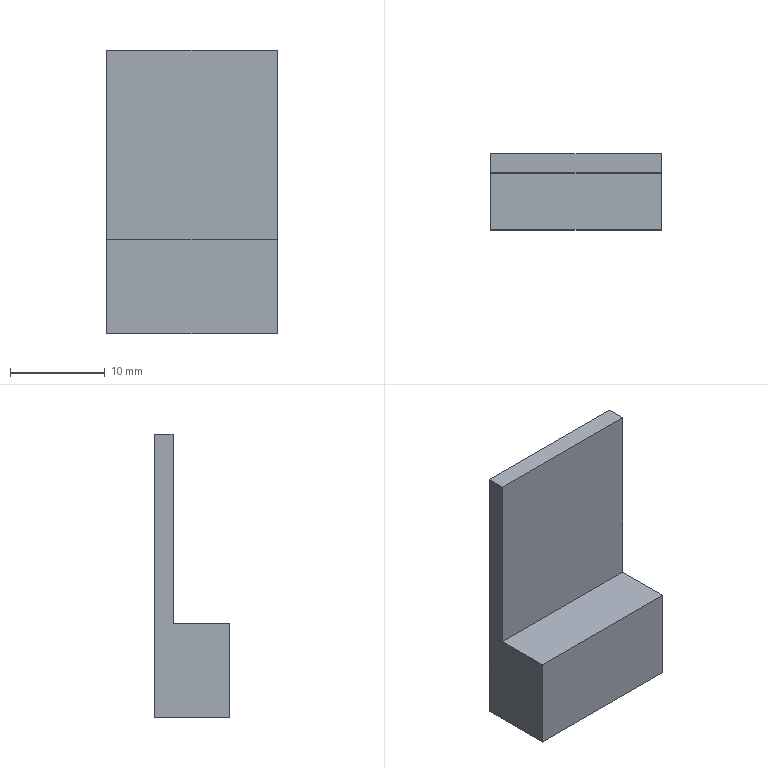Part | SolidWorks | features 3DProfileFeature 1, Extrusion 1, HoleWzd 1, ICE 1, MirrorPattern 1 | 1 solid | 20 faces | box 18 x 8 x 30 mm | volume 2093 mm3 | cone 8 | plane 8 | cylinder 4 | commonest cylinder face diameters 2.5 x4
STEP:
#1=CARTESIAN_POINT('',(-3.75,0.,0.275));
#2=VERTEX_POINT('',#1);
#3=CARTESIAN_POINT('',(-6.25,0.,0.275));
#4=VERTEX_POINT('',#3);
#5=CARTESIAN_POINT('',(-5.,0.,0.275));
#6=DIRECTION('',(0.,0.,-1.));
#7=DIRECTION('',(-1.,0.,0.));
#8=AXIS2_PLACEMENT_3D('',#5,#6,#7);
#9=CIRCLE('',#8,1.25);
#10=EDGE_CURVE('',#2,#4,#9,.T.);
#11=ORIENTED_EDGE('',*,*,#10,.F.);
#12=CARTESIAN_POINT('',(-3.475,0.,0.));
#13=VERTEX_POINT('',#12);
#14=CARTESIAN_POINT('',(-3.475,0.,0.));
#15=DIRECTION('',(0.7071,0.,-0.7071));
#16=VECTOR('',#15,1000.);
#17=LINE('',#14,#16);
#18=EDGE_CURVE('',#2,#13,#17,.T.);
#19=ORIENTED_EDGE('',*,*,#18,.T.);
#20=CARTESIAN_POINT('',(-6.525,0.,0.));
#21=VERTEX_POINT('',#20);
#22=CARTESIAN_POINT('',(-5.,0.,0.));
#23=DIRECTION('',(0.,0.,-1.));
#24=DIRECTION('',(-1.,0.,0.));
#25=AXIS2_PLACEMENT_3D('',#22,#23,#24);
#26=CIRCLE('',#25,1.525);
#27=EDGE_CURVE('',#13,#21,#26,.T.);
#28=ORIENTED_EDGE('',*,*,#27,.T.);
#29=CARTESIAN_POINT('',(-6.525,0.,0.));
#30=DIRECTION('',(-0.7071,0.,-0.7071));
#31=VECTOR('',#30,1000.);
#32=LINE('',#29,#31);
#33=EDGE_CURVE('',#4,#21,#32,.T.);
#34=ORIENTED_EDGE('',*,*,#33,.F.);
#35=EDGE_LOOP('',(#11,#19,#28,#34));
#36=FACE_OUTER_BOUND('',#35,.T.);
#37=CARTESIAN_POINT('',(-5.,0.,0.));
#38=DIRECTION('',(0.,0.,-1.));
#39=DIRECTION('',(-1.,0.,0.));
#40=AXIS2_PLACEMENT_3D('',#37,#38,#39);
#41=CONICAL_SURFACE('',#40,1.525,0.7854);
#42=ADVANCED_FACE('',(#36),#41,.F.);
#43=CARTESIAN_POINT('',(-3.75,0.,6.5));
#44=VERTEX_POINT('',#43);
#45=CARTESIAN_POINT('',(-6.25,0.,6.5));
#46=VERTEX_POINT('',#45);
#47=CARTESIAN_POINT('',(-5.,0.,6.5));
#48=DIRECTION('',(0.,0.,-1.));
#49=DIRECTION('',(-1.,0.,0.));
#50=AXIS2_PLACEMENT_3D('',#47,#48,#49);
#51=CIRCLE('',#50,1.25);
#52=EDGE_CURVE('',#44,#46,#51,.T.);
#53=ORIENTED_EDGE('',*,*,#52,.F.);
#54=CARTESIAN_POINT('',(-3.75,0.,0.));
#55=DIRECTION('',(0.,0.,-1.));
#56=VECTOR('',#55,1000.);
#57=LINE('',#54,#56);
#58=EDGE_CURVE('',#44,#2,#57,.T.);
#59=ORIENTED_EDGE('',*,*,#58,.T.);
#60=ORIENTED_EDGE('',*,*,#10,.T.);
#61=CARTESIAN_POINT('',(-6.25,0.,0.));
#62=DIRECTION('',(0.,0.,-1.));
#63=VECTOR('',#62,1000.);
#64=LINE('',#61,#63);
#65=EDGE_CURVE('',#46,#4,#64,.T.);
#66=ORIENTED_EDGE('',*,*,#65,.F.);
#67=EDGE_LOOP('',(#53,#59,#60,#66));
#68=FACE_OUTER_BOUND('',#67,.T.);
#69=CARTESIAN_POINT('',(-5.,0.,0.));
#70=DIRECTION('',(0.,0.,-1.));
#71=DIRECTION('',(-1.,0.,0.));
#72=AXIS2_PLACEMENT_3D('',#69,#70,#71);
#73=CYLINDRICAL_SURFACE('',#72,1.25);
#74=ADVANCED_FACE('',(#68),#73,.F.);
#75=CARTESIAN_POINT('',(-5.,0.,7.251));
#76=VERTEX_POINT('',#75);
#77=CARTESIAN_POINT('',(-6.25,0.,6.5));
#78=DIRECTION('',(-0.8572,0.,-0.515));
#79=VECTOR('',#78,1000.);
#80=LINE('',#77,#79);
#81=EDGE_CURVE('',#76,#46,#80,.T.);
#82=ORIENTED_EDGE('',*,*,#81,.F.);
#83=CARTESIAN_POINT('',(-3.75,0.,6.5));
#84=DIRECTION('',(0.8572,0.,-0.515));
#85=VECTOR('',#84,1000.);
#86=LINE('',#83,#85);
#87=EDGE_CURVE('',#76,#44,#86,.T.);
#88=ORIENTED_EDGE('',*,*,#87,.T.);
#89=ORIENTED_EDGE('',*,*,#52,.T.);
#90=EDGE_LOOP('',(#82,#88,#89));
#91=FACE_OUTER_BOUND('',#90,.T.);
#92=CARTESIAN_POINT('',(-5.,0.,6.5));
#93=DIRECTION('',(0.,0.,-1.));
#94=DIRECTION('',(-1.,0.,0.));
#95=AXIS2_PLACEMENT_3D('',#92,#93,#94);
#96=CONICAL_SURFACE('',#95,1.25,1.03);
#97=ADVANCED_FACE('',(#91),#96,.F.);
#98=CARTESIAN_POINT('',(6.25,0.,0.275));
#99=VERTEX_POINT('',#98);
#100=CARTESIAN_POINT('',(3.75,0.,0.275));
#101=VERTEX_POINT('',#100);
#102=CARTESIAN_POINT('',(5.,0.,0.275));
#103=DIRECTION('',(0.,0.,-1.));
#104=DIRECTION('',(-1.,0.,0.));
#105=AXIS2_PLACEMENT_3D('',#102,#103,#104);
#106=CIRCLE('',#105,1.25);
#107=EDGE_CURVE('',#99,#101,#106,.T.);
#108=ORIENTED_EDGE('',*,*,#107,.F.);
#109=CARTESIAN_POINT('',(6.525,0.,0.));
#110=VERTEX_POINT('',#109);
#111=CARTESIAN_POINT('',(6.525,0.,0.));
#112=DIRECTION('',(0.7071,0.,-0.7071));
#113=VECTOR('',#112,1000.);
#114=LINE('',#111,#113);
#115=EDGE_CURVE('',#99,#110,#114,.T.);
#116=ORIENTED_EDGE('',*,*,#115,.T.);
#117=CARTESIAN_POINT('',(3.475,0.,0.));
#118=VERTEX_POINT('',#117);
#119=CARTESIAN_POINT('',(5.,0.,0.));
#120=DIRECTION('',(0.,0.,-1.));
#121=DIRECTION('',(-1.,0.,0.));
#122=AXIS2_PLACEMENT_3D('',#119,#120,#121);
#123=CIRCLE('',#122,1.525);
#124=EDGE_CURVE('',#110,#118,#123,.T.);
#125=ORIENTED_EDGE('',*,*,#124,.T.);
#126=CARTESIAN_POINT('',(3.475,0.,0.));
#127=DIRECTION('',(-0.7071,0.,-0.7071));
#128=VECTOR('',#127,1000.);
#129=LINE('',#126,#128);
#130=EDGE_CURVE('',#101,#118,#129,.T.);
#131=ORIENTED_EDGE('',*,*,#130,.F.);
#132=EDGE_LOOP('',(#108,#116,#125,#131));
#133=FACE_OUTER_BOUND('',#132,.T.);
#134=CARTESIAN_POINT('',(5.,0.,0.));
#135=DIRECTION('',(0.,0.,-1.));
#136=DIRECTION('',(-1.,0.,0.));
#137=AXIS2_PLACEMENT_3D('',#134,#135,#136);
#138=CONICAL_SURFACE('',#137,1.525,0.7854);
#139=ADVANCED_FACE('',(#133),#138,.F.);
#140=CARTESIAN_POINT('',(6.25,0.,6.5));
#141=VERTEX_POINT('',#140);
#142=CARTESIAN_POINT('',(3.75,0.,6.5));
#143=VERTEX_POINT('',#142);
#144=CARTESIAN_POINT('',(5.,0.,6.5));
#145=DIRECTION('',(0.,0.,-1.));
#146=DIRECTION('',(-1.,0.,0.));
#147=AXIS2_PLACEMENT_3D('',#144,#145,#146);
#148=CIRCLE('',#147,1.25);
#149=EDGE_CURVE('',#141,#143,#148,.T.);
#150=ORIENTED_EDGE('',*,*,#149,.F.);
#151=CARTESIAN_POINT('',(6.25,0.,0.));
#152=DIRECTION('',(0.,0.,-1.));
#153=VECTOR('',#152,1000.);
#154=LINE('',#151,#153);
#155=EDGE_CURVE('',#141,#99,#154,.T.);
#156=ORIENTED_EDGE('',*,*,#155,.T.);
#157=ORIENTED_EDGE('',*,*,#107,.T.);
#158=CARTESIAN_POINT('',(3.75,0.,0.));
#159=DIRECTION('',(0.,0.,-1.));
#160=VECTOR('',#159,1000.);
#161=LINE('',#158,#160);
#162=EDGE_CURVE('',#143,#101,#161,.T.);
#163=ORIENTED_EDGE('',*,*,#162,.F.);
#164=EDGE_LOOP('',(#150,#156,#157,#163));
#165=FACE_OUTER_BOUND('',#164,.T.);
#166=CARTESIAN_POINT('',(5.,0.,0.));
#167=DIRECTION('',(0.,0.,-1.));
#168=DIRECTION('',(-1.,0.,0.));
#169=AXIS2_PLACEMENT_3D('',#166,#167,#168);
#170=CYLINDRICAL_SURFACE('',#169,1.25);
#171=ADVANCED_FACE('',(#165),#170,.F.);
#172=CARTESIAN_POINT('',(5.,0.,7.251));
#173=VERTEX_POINT('',#172);
#174=CARTESIAN_POINT('',(3.75,0.,6.5));
#175=DIRECTION('',(-0.8572,0.,-0.515));
#176=VECTOR('',#175,1000.);
#177=LINE('',#174,#176);
#178=EDGE_CURVE('',#173,#143,#177,.T.);
#179=ORIENTED_EDGE('',*,*,#178,.F.);
#180=CARTESIAN_POINT('',(6.25,0.,6.5));
#181=DIRECTION('',(0.8572,0.,-0.515));
#182=VECTOR('',#181,1000.);
#183=LINE('',#180,#182);
#184=EDGE_CURVE('',#173,#141,#183,.T.);
#185=ORIENTED_EDGE('',*,*,#184,.T.);
#186=ORIENTED_EDGE('',*,*,#149,.T.);
#187=EDGE_LOOP('',(#179,#185,#186));
#188=FACE_OUTER_BOUND('',#187,.T.);
#189=CARTESIAN_POINT('',(5.,0.,6.5));
#190=DIRECTION('',(0.,0.,-1.));
#191=DIRECTION('',(-1.,0.,0.));
#192=AXIS2_PLACEMENT_3D('',#189,#190,#191);
#193=CONICAL_SURFACE('',#192,1.25,1.03);
#194=ADVANCED_FACE('',(#188),#193,.F.);
#195=CARTESIAN_POINT('',(-9.,2.,10.));
#196=VERTEX_POINT('',#195);
#197=CARTESIAN_POINT('',(9.,2.,10.));
#198=VERTEX_POINT('',#197);
#199=CARTESIAN_POINT('',(-9.,2.,10.));
#200=DIRECTION('',(1.,0.,0.));
#201=VECTOR('',#200,1000.);
#202=LINE('',#199,#201);
#203=EDGE_CURVE('',#196,#198,#202,.T.);
#204=ORIENTED_EDGE('',*,*,#203,.F.);
#205=CARTESIAN_POINT('',(-9.,-4.,10.));
#206=VERTEX_POINT('',#205);
#207=CARTESIAN_POINT('',(-9.,-4.,10.));
#208=DIRECTION('',(0.,-1.,0.));
#209=VECTOR('',#208,1000.);
#210=LINE('',#207,#209);
#211=EDGE_CURVE('',#196,#206,#210,.T.);
#212=ORIENTED_EDGE('',*,*,#211,.T.);
#213=CARTESIAN_POINT('',(9.,-4.,10.));
#214=VERTEX_POINT('',#213);
#215=CARTESIAN_POINT('',(-9.,-4.,10.));
#216=DIRECTION('',(1.,0.,0.));
#217=VECTOR('',#216,1000.);
#218=LINE('',#215,#217);
#219=EDGE_CURVE('',#206,#214,#218,.T.);
#220=ORIENTED_EDGE('',*,*,#219,.T.);
#221=CARTESIAN_POINT('',(9.,-4.,10.));
#222=DIRECTION('',(0.,1.,0.));
#223=VECTOR('',#222,1000.);
#224=LINE('',#221,#223);
#225=EDGE_CURVE('',#214,#198,#224,.T.);
#226=ORIENTED_EDGE('',*,*,#225,.T.);
#227=EDGE_LOOP('',(#204,#212,#220,#226));
#228=FACE_OUTER_BOUND('',#227,.T.);
#229=CARTESIAN_POINT('',(0.,0.,10.));
#230=DIRECTION('',(0.,0.,-1.));
#231=DIRECTION('',(-1.,0.,0.));
#232=AXIS2_PLACEMENT_3D('',#229,#230,#231);
#233=PLANE('',#232);
#234=ADVANCED_FACE('',(#228),#233,.F.);
#235=CARTESIAN_POINT('',(9.,-4.,0.));
#236=VERTEX_POINT('',#235);
#237=CARTESIAN_POINT('',(9.,4.,0.));
#238=VERTEX_POINT('',#237);
#239=CARTESIAN_POINT('',(9.,-4.,0.));
#240=DIRECTION('',(0.,1.,0.));
#241=VECTOR('',#240,1000.);
#242=LINE('',#239,#241);
#243=EDGE_CURVE('',#236,#238,#242,.T.);
#244=ORIENTED_EDGE('',*,*,#243,.T.);
#245=CARTESIAN_POINT('',(9.,4.,30.));
#246=VERTEX_POINT('',#245);
#247=CARTESIAN_POINT('',(9.,4.,10.));
#248=DIRECTION('',(0.,0.,-1.));
#249=VECTOR('',#248,1000.);
#250=LINE('',#247,#249);
#251=EDGE_CURVE('',#246,#238,#250,.T.);
#252=ORIENTED_EDGE('',*,*,#251,.F.);
#253=CARTESIAN_POINT('',(9.,2.,30.));
#254=VERTEX_POINT('',#253);
#255=CARTESIAN_POINT('',(9.,4.,30.));
#256=DIRECTION('',(0.,1.,0.));
#257=VECTOR('',#256,1000.);
#258=LINE('',#255,#257);
#259=EDGE_CURVE('',#254,#246,#258,.T.);
#260=ORIENTED_EDGE('',*,*,#259,.F.);
#261=CARTESIAN_POINT('',(9.,2.,30.));
#262=DIRECTION('',(0.,0.,-1.));
#263=VECTOR('',#262,1000.);
#264=LINE('',#261,#263);
#265=EDGE_CURVE('',#254,#198,#264,.T.);
#266=ORIENTED_EDGE('',*,*,#265,.T.);
#267=ORIENTED_EDGE('',*,*,#225,.F.);
#268=CARTESIAN_POINT('',(9.,-4.,10.));
#269=DIRECTION('',(0.,0.,-1.));
#270=VECTOR('',#269,1000.);
#271=LINE('',#268,#270);
#272=EDGE_CURVE('',#214,#236,#271,.T.);
#273=ORIENTED_EDGE('',*,*,#272,.T.);
#274=EDGE_LOOP('',(#244,#252,#260,#266,#267,#273));
#275=FACE_OUTER_BOUND('',#274,.T.);
#276=CARTESIAN_POINT('',(9.,-4.,10.));
#277=DIRECTION('',(-1.,0.,0.));
#278=DIRECTION('',(0.,0.,1.));
#279=AXIS2_PLACEMENT_3D('',#276,#277,#278);
#280=PLANE('',#279);
#281=ADVANCED_FACE('',(#275),#280,.F.);
#282=CARTESIAN_POINT('',(-9.,4.,0.));
#283=VERTEX_POINT('',#282);
#284=CARTESIAN_POINT('',(-9.,4.,0.));
#285=DIRECTION('',(-1.,0.,0.));
#286=VECTOR('',#285,1000.);
#287=LINE('',#284,#286);
#288=EDGE_CURVE('',#238,#283,#287,.T.);
#289=ORIENTED_EDGE('',*,*,#288,.T.);
#290=CARTESIAN_POINT('',(-9.,4.,30.));
#291=VERTEX_POINT('',#290);
#292=CARTESIAN_POINT('',(-9.,4.,10.));
#293=DIRECTION('',(0.,0.,-1.));
#294=VECTOR('',#293,1000.);
#295=LINE('',#292,#294);
#296=EDGE_CURVE('',#291,#283,#295,.T.);
#297=ORIENTED_EDGE('',*,*,#296,.F.);
#298=CARTESIAN_POINT('',(-9.,4.,30.));
#299=DIRECTION('',(-1.,0.,0.));
#300=VECTOR('',#299,1000.);
#301=LINE('',#298,#300);
#302=EDGE_CURVE('',#246,#291,#301,.T.);
#303=ORIENTED_EDGE('',*,*,#302,.F.);
#304=ORIENTED_EDGE('',*,*,#251,.T.);
#305=EDGE_LOOP('',(#289,#297,#303,#304));
#306=FACE_OUTER_BOUND('',#305,.T.);
#307=CARTESIAN_POINT('',(-9.,4.,10.));
#308=DIRECTION('',(0.,-1.,0.));
#309=DIRECTION('',(0.,0.,-1.));
#310=AXIS2_PLACEMENT_3D('',#307,#308,#309);
#311=PLANE('',#310);
#312=ADVANCED_FACE('',(#306),#311,.F.);
#313=CARTESIAN_POINT('',(-9.,-4.,0.));
#314=VERTEX_POINT('',#313);
#315=CARTESIAN_POINT('',(-9.,-4.,0.));
#316=DIRECTION('',(0.,-1.,0.));
#317=VECTOR('',#316,1000.);
#318=LINE('',#315,#317);
#319=EDGE_CURVE('',#283,#314,#318,.T.);
#320=ORIENTED_EDGE('',*,*,#319,.T.);
#321=CARTESIAN_POINT('',(-9.,-4.,10.));
#322=DIRECTION('',(0.,0.,-1.));
#323=VECTOR('',#322,1000.);
#324=LINE('',#321,#323);
#325=EDGE_CURVE('',#206,#314,#324,.T.);
#326=ORIENTED_EDGE('',*,*,#325,.F.);
#327=ORIENTED_EDGE('',*,*,#211,.F.);
#328=CARTESIAN_POINT('',(-9.,2.,30.));
#329=VERTEX_POINT('',#328);
#330=CARTESIAN_POINT('',(-9.,2.,30.));
#331=DIRECTION('',(0.,0.,-1.));
#332=VECTOR('',#331,1000.);
#333=LINE('',#330,#332);
#334=EDGE_CURVE('',#329,#196,#333,.T.);
#335=ORIENTED_EDGE('',*,*,#334,.F.);
#336=CARTESIAN_POINT('',(-9.,4.,30.));
#337=DIRECTION('',(0.,-1.,0.));
#338=VECTOR('',#337,1000.);
#339=LINE('',#336,#338);
#340=EDGE_CURVE('',#291,#329,#339,.T.);
#341=ORIENTED_EDGE('',*,*,#340,.F.);
#342=ORIENTED_EDGE('',*,*,#296,.T.);
#343=EDGE_LOOP('',(#320,#326,#327,#335,#341,#342));
#344=FACE_OUTER_BOUND('',#343,.T.);
#345=CARTESIAN_POINT('',(-9.,-4.,10.));
#346=DIRECTION('',(1.,0.,0.));
#347=DIRECTION('',(0.,0.,-1.));
#348=AXIS2_PLACEMENT_3D('',#345,#346,#347);
#349=PLANE('',#348);
#350=ADVANCED_FACE('',(#344),#349,.F.);
#351=CARTESIAN_POINT('',(-9.,-4.,0.));
#352=DIRECTION('',(1.,0.,0.));
#353=VECTOR('',#352,1000.);
#354=LINE('',#351,#353);
#355=EDGE_CURVE('',#314,#236,#354,.T.);
#356=ORIENTED_EDGE('',*,*,#355,.T.);
#357=ORIENTED_EDGE('',*,*,#272,.F.);
#358=ORIENTED_EDGE('',*,*,#219,.F.);
#359=ORIENTED_EDGE('',*,*,#325,.T.);
#360=EDGE_LOOP('',(#356,#357,#358,#359));
#361=FACE_OUTER_BOUND('',#360,.T.);
#362=CARTESIAN_POINT('',(-9.,-4.,10.));
#363=DIRECTION('',(0.,1.,0.));
#364=DIRECTION('',(0.,0.,1.));
#365=AXIS2_PLACEMENT_3D('',#362,#363,#364);
#366=PLANE('',#365);
#367=ADVANCED_FACE('',(#361),#366,.F.);
#368=CARTESIAN_POINT('',(-5.,0.,0.));
#369=DIRECTION('',(0.,0.,-1.));
#370=DIRECTION('',(-1.,0.,0.));
#371=AXIS2_PLACEMENT_3D('',#368,#369,#370);
#372=CIRCLE('',#371,1.525);
#373=EDGE_CURVE('',#21,#13,#372,.T.);
#374=ORIENTED_EDGE('',*,*,#373,.F.);
#375=ORIENTED_EDGE('',*,*,#27,.F.);
#376=EDGE_LOOP('',(#374,#375));
#377=FACE_BOUND('',#376,.T.);
#378=CARTESIAN_POINT('',(5.,0.,0.));
#379=DIRECTION('',(0.,0.,-1.));
#380=DIRECTION('',(-1.,0.,0.));
#381=AXIS2_PLACEMENT_3D('',#378,#379,#380);
#382=CIRCLE('',#381,1.525);
#383=EDGE_CURVE('',#118,#110,#382,.T.);
#384=ORIENTED_EDGE('',*,*,#383,.F.);
#385=ORIENTED_EDGE('',*,*,#124,.F.);
#386=EDGE_LOOP('',(#384,#385));
#387=FACE_BOUND('',#386,.T.);
#388=ORIENTED_EDGE('',*,*,#243,.F.);
#389=ORIENTED_EDGE('',*,*,#355,.F.);
#390=ORIENTED_EDGE('',*,*,#319,.F.);
#391=ORIENTED_EDGE('',*,*,#288,.F.);
#392=EDGE_LOOP('',(#388,#389,#390,#391));
#393=FACE_OUTER_BOUND('',#392,.T.);
#394=CARTESIAN_POINT('',(0.,0.,0.));
#395=DIRECTION('',(0.,0.,-1.));
#396=DIRECTION('',(-1.,0.,0.));
#397=AXIS2_PLACEMENT_3D('',#394,#395,#396);
#398=PLANE('',#397);
#399=ADVANCED_FACE('',(#377,#387,#393),#398,.T.);
#400=ORIENTED_EDGE('',*,*,#203,.T.);
#401=ORIENTED_EDGE('',*,*,#265,.F.);
#402=CARTESIAN_POINT('',(-9.,2.,30.));
#403=DIRECTION('',(1.,0.,0.));
#404=VECTOR('',#403,1000.);
#405=LINE('',#402,#404);
#406=EDGE_CURVE('',#329,#254,#405,.T.);
#407=ORIENTED_EDGE('',*,*,#406,.F.);
#408=ORIENTED_EDGE('',*,*,#334,.T.);
#409=EDGE_LOOP('',(#400,#401,#407,#408));
#410=FACE_OUTER_BOUND('',#409,.T.);
#411=CARTESIAN_POINT('',(-9.,2.,30.));
#412=DIRECTION('',(0.,1.,0.));
#413=DIRECTION('',(0.,0.,1.));
#414=AXIS2_PLACEMENT_3D('',#411,#412,#413);
#415=PLANE('',#414);
#416=ADVANCED_FACE('',(#410),#415,.F.);
#417=ORIENTED_EDGE('',*,*,#340,.T.);
#418=ORIENTED_EDGE('',*,*,#406,.T.);
#419=ORIENTED_EDGE('',*,*,#259,.T.);
#420=ORIENTED_EDGE('',*,*,#302,.T.);
#421=EDGE_LOOP('',(#417,#418,#419,#420));
#422=FACE_OUTER_BOUND('',#421,.T.);
#423=CARTESIAN_POINT('',(0.,0.,30.));
#424=DIRECTION('',(0.,0.,1.));
#425=DIRECTION('',(1.,0.,0.));
#426=AXIS2_PLACEMENT_3D('',#423,#424,#425);
#427=PLANE('',#426);
#428=ADVANCED_FACE('',(#422),#427,.T.);
#429=ORIENTED_EDGE('',*,*,#184,.F.);
#430=ORIENTED_EDGE('',*,*,#178,.T.);
#431=CARTESIAN_POINT('',(5.,0.,6.5));
#432=DIRECTION('',(0.,0.,-1.));
#433=DIRECTION('',(-1.,0.,0.));
#434=AXIS2_PLACEMENT_3D('',#431,#432,#433);
#435=CIRCLE('',#434,1.25);
#436=EDGE_CURVE('',#143,#141,#435,.T.);
#437=ORIENTED_EDGE('',*,*,#436,.T.);
#438=EDGE_LOOP('',(#429,#430,#437));
#439=FACE_OUTER_BOUND('',#438,.T.);
#440=CARTESIAN_POINT('',(5.,0.,6.5));
#441=DIRECTION('',(0.,0.,-1.));
#442=DIRECTION('',(-1.,0.,0.));
#443=AXIS2_PLACEMENT_3D('',#440,#441,#442);
#444=CONICAL_SURFACE('',#443,1.25,1.03);
#445=ADVANCED_FACE('',(#439),#444,.F.);
#446=ORIENTED_EDGE('',*,*,#155,.F.);
#447=ORIENTED_EDGE('',*,*,#436,.F.);
#448=ORIENTED_EDGE('',*,*,#162,.T.);
#449=CARTESIAN_POINT('',(5.,0.,0.275));
#450=DIRECTION('',(0.,0.,-1.));
#451=DIRECTION('',(-1.,0.,0.));
#452=AXIS2_PLACEMENT_3D('',#449,#450,#451);
#453=CIRCLE('',#452,1.25);
#454=EDGE_CURVE('',#101,#99,#453,.T.);
#455=ORIENTED_EDGE('',*,*,#454,.T.);
#456=EDGE_LOOP('',(#446,#447,#448,#455));
#457=FACE_OUTER_BOUND('',#456,.T.);
#458=CARTESIAN_POINT('',(5.,0.,0.));
#459=DIRECTION('',(0.,0.,-1.));
#460=DIRECTION('',(-1.,0.,0.));
#461=AXIS2_PLACEMENT_3D('',#458,#459,#460);
#462=CYLINDRICAL_SURFACE('',#461,1.25);
#463=ADVANCED_FACE('',(#457),#462,.F.);
#464=ORIENTED_EDGE('',*,*,#115,.F.);
#465=ORIENTED_EDGE('',*,*,#454,.F.);
#466=ORIENTED_EDGE('',*,*,#130,.T.);
#467=ORIENTED_EDGE('',*,*,#383,.T.);
#468=EDGE_LOOP('',(#464,#465,#466,#467));
#469=FACE_OUTER_BOUND('',#468,.T.);
#470=CARTESIAN_POINT('',(5.,0.,0.));
#471=DIRECTION('',(0.,0.,-1.));
#472=DIRECTION('',(-1.,0.,0.));
#473=AXIS2_PLACEMENT_3D('',#470,#471,#472);
#474=CONICAL_SURFACE('',#473,1.525,0.7854);
#475=ADVANCED_FACE('',(#469),#474,.F.);
#476=ORIENTED_EDGE('',*,*,#87,.F.);
#477=ORIENTED_EDGE('',*,*,#81,.T.);
#478=CARTESIAN_POINT('',(-5.,0.,6.5));
#479=DIRECTION('',(0.,0.,-1.));
#480=DIRECTION('',(-1.,0.,0.));
#481=AXIS2_PLACEMENT_3D('',#478,#479,#480);
#482=CIRCLE('',#481,1.25);
#483=EDGE_CURVE('',#46,#44,#482,.T.);
#484=ORIENTED_EDGE('',*,*,#483,.T.);
#485=EDGE_LOOP('',(#476,#477,#484));
#486=FACE_OUTER_BOUND('',#485,.T.);
#487=CARTESIAN_POINT('',(-5.,0.,6.5));
#488=DIRECTION('',(0.,0.,-1.));
#489=DIRECTION('',(-1.,0.,0.));
#490=AXIS2_PLACEMENT_3D('',#487,#488,#489);
#491=CONICAL_SURFACE('',#490,1.25,1.03);
#492=ADVANCED_FACE('',(#486),#491,.F.);
#493=ORIENTED_EDGE('',*,*,#58,.F.);
#494=ORIENTED_EDGE('',*,*,#483,.F.);
#495=ORIENTED_EDGE('',*,*,#65,.T.);
#496=CARTESIAN_POINT('',(-5.,0.,0.275));
#497=DIRECTION('',(0.,0.,-1.));
#498=DIRECTION('',(-1.,0.,0.));
#499=AXIS2_PLACEMENT_3D('',#496,#497,#498);
#500=CIRCLE('',#499,1.25);
#501=EDGE_CURVE('',#4,#2,#500,.T.);
#502=ORIENTED_EDGE('',*,*,#501,.T.);
#503=EDGE_LOOP('',(#493,#494,#495,#502));
#504=FACE_OUTER_BOUND('',#503,.T.);
#505=CARTESIAN_POINT('',(-5.,0.,0.));
#506=DIRECTION('',(0.,0.,-1.));
#507=DIRECTION('',(-1.,0.,0.));
#508=AXIS2_PLACEMENT_3D('',#505,#506,#507);
#509=CYLINDRICAL_SURFACE('',#508,1.25);
#510=ADVANCED_FACE('',(#504),#509,.F.);
#511=ORIENTED_EDGE('',*,*,#18,.F.);
#512=ORIENTED_EDGE('',*,*,#501,.F.);
#513=ORIENTED_EDGE('',*,*,#33,.T.);
#514=ORIENTED_EDGE('',*,*,#373,.T.);
#515=EDGE_LOOP('',(#511,#512,#513,#514));
#516=FACE_OUTER_BOUND('',#515,.T.);
#517=CARTESIAN_POINT('',(-5.,0.,0.));
#518=DIRECTION('',(0.,0.,-1.));
#519=DIRECTION('',(-1.,0.,0.));
#520=AXIS2_PLACEMENT_3D('',#517,#518,#519);
#521=CONICAL_SURFACE('',#520,1.525,0.7854);
#522=ADVANCED_FACE('',(#516),#521,.F.);
#523=CLOSED_SHELL('',(#42,#74,#97,#139,#171,#194,#234,#281,#312,#350,#367,#399,#416,#428,#445,#463,#475,#492,#510,#522));
#524=MANIFOLD_SOLID_BREP('',#523);
#525=CARTESIAN_POINT('',(0.,0.,0.));
#526=DIRECTION('',(0.,0.,1.));
#527=DIRECTION('',(1.,0.,0.));
#528=AXIS2_PLACEMENT_3D('',#525,#526,#527);
#529=(LENGTH_UNIT()NAMED_UNIT(*)SI_UNIT(.MILLI.,.METRE.));
#530=UNCERTAINTY_MEASURE_WITH_UNIT(LENGTH_MEASURE(0.00001),#529,'','');
#531=(NAMED_UNIT(*)PLANE_ANGLE_UNIT()SI_UNIT($,.RADIAN.));
#532=(NAMED_UNIT(*)SI_UNIT($,.STERADIAN.)SOLID_ANGLE_UNIT());
#533=(GEOMETRIC_REPRESENTATION_CONTEXT(3)GLOBAL_UNCERTAINTY_ASSIGNED_CONTEXT((#530))GLOBAL_UNIT_ASSIGNED_CONTEXT((#529,#531,#532))REPRESENTATION_CONTEXT('',''));
#534=ADVANCED_BREP_SHAPE_REPRESENTATION('',(#524,#528),#533);